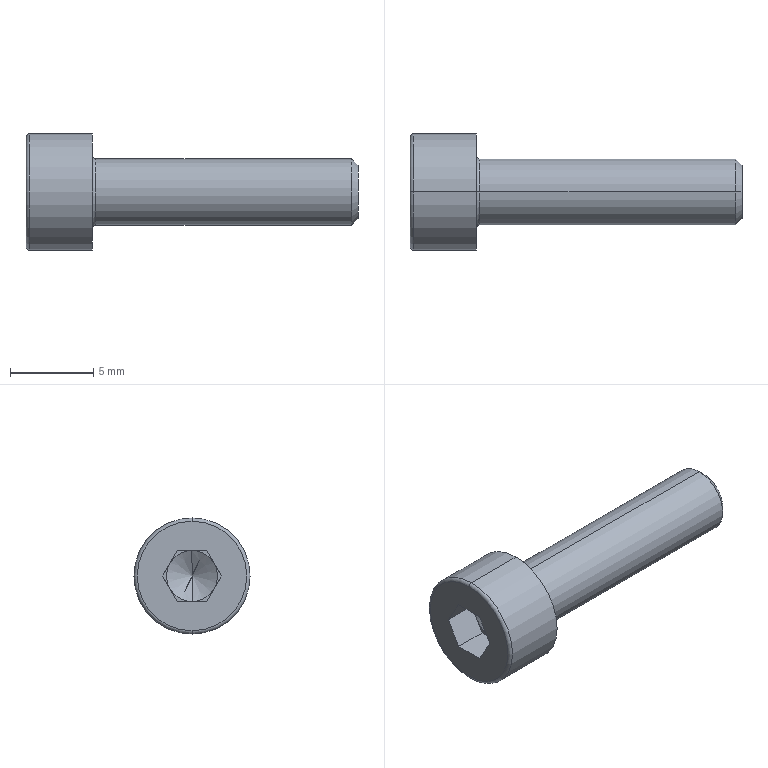Part | STEP file | socket head cap screw_iso_ISO 4762 M4 x 16 --- 16N | 1 solid | 27 faces | box 20 x 7 x 7 mm | volume 335.506 mm3 | plane 15 | cone 4 | torus 4 | cylinder 4 | commonest cylinder face diameters 4 x2 7 x2